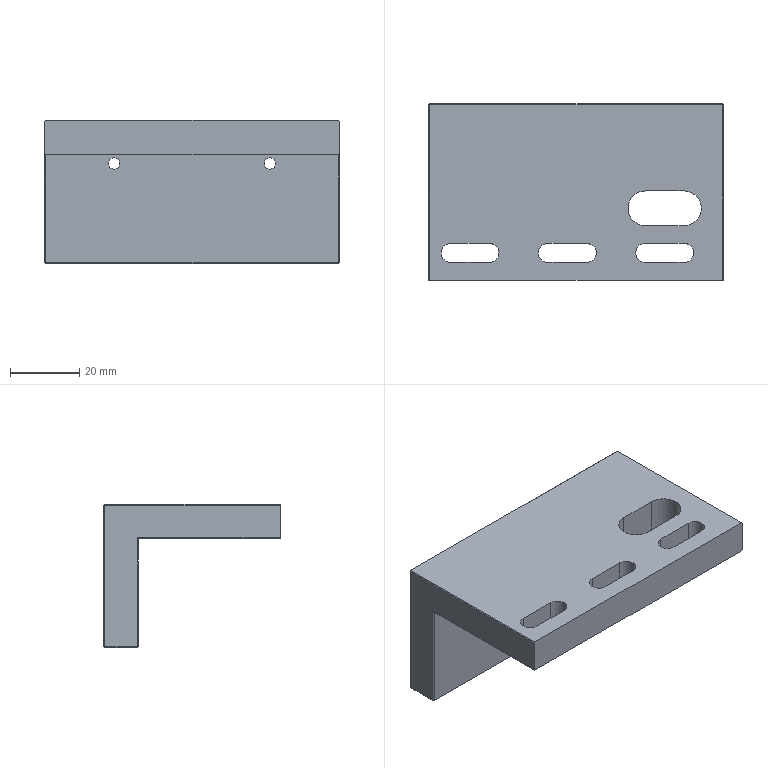Part | NX | 1 solid | 65 faces | box 85 x 51 x 41.5 mm | volume 65353 mm3 | plane 29 | cylinder 24 | cone 12 | commonest cylinder face diameters 5.5 x9 2.5 x8 3.3 x4 10 x3